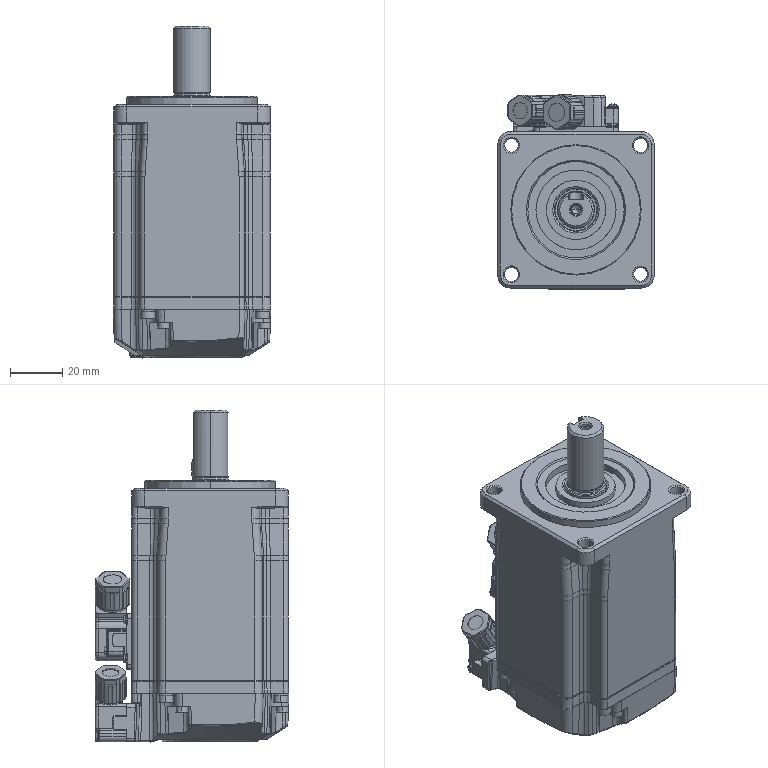Part | SolidWorks | features BaseBody 3 | 3 solids | 3195 faces | volume 325247 mm3 | plane 1352 | cylinder 889 | spline 771 | cone 183 | commonest cylinder face diameters 0.4 x159 0.6 x106 4 x82 1 x73 2 x60 0.3 x54